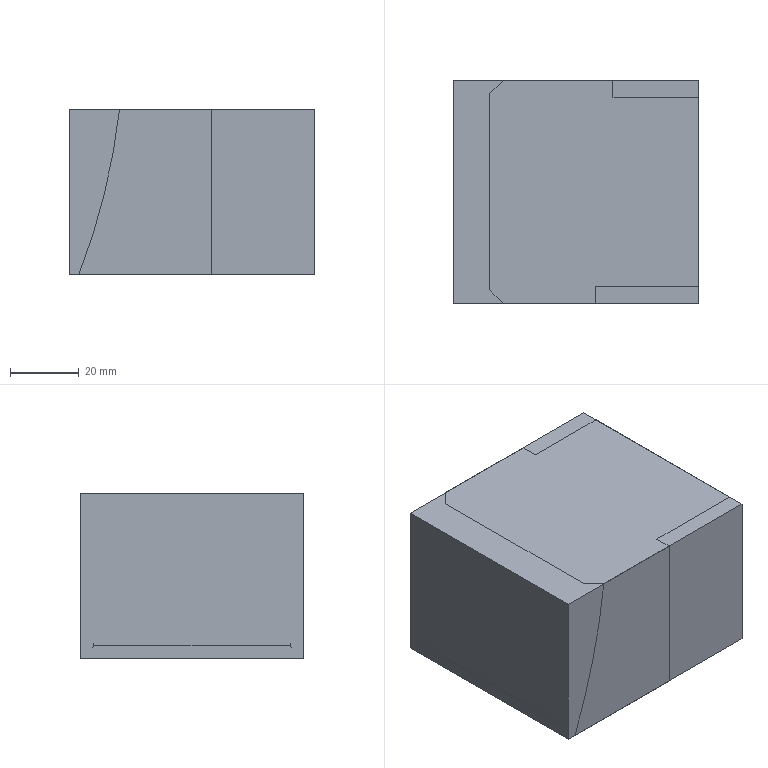NC program | NX | posted with a generic post | part box 71.51 x 65 x 48 mm
Whole program:
N10 G17 G21 G94 G90
(DRILLING_COPY_1 , TOOL : D6A45)
N12 T07 M6
N14 G54
N16 G17 G0 G90 X20. Y-16. B0. C0. S5000 M3
N18 G43 Z30. H7
N20 G94 G81 G98 Z-1. F250. R3.
N22 Y0.
N24 Y16.
N26 X-20.
N28 Y0.
N30 Y-16.
N32 G80
N34 G0 X-20. Y-16. Z30.
N36 M5
(DRILLING_COPY_COPY_1 , TOOL : 4.8ZT)
N38 T14 M6
N40 G54
N42 G17 G0 G90 X20. Y0. B0. C0. S2000 M3
N44 G43 Z30. H14
N46 G94 G83 G98 Z-13.442 F120. Q2. R3.
N48 X-20.
N50 G80
N52 G0 X-20. Y0. Z30.
N54 M5
(DRILLING_COPY_COPY_1_COPY , TOOL : 5.0JD)
N56 T15 M6
N58 G54
N60 G17 G0 G90 X20. Y0. B0. C0. S1000 M3
N62 G43 Z30. H15
N64 G94 G85 G98 Z-12. F50. R3.
N66 X-20.
N68 G80
N70 G0 X-20. Y0. Z30.
N72 M5
(DRILLING_COPY_COPY_1_COPY_1 , TOOL : 7.0ZT)
N74 T17 M6
N76 G54
N78 G17 G0 G90 X20. Y-16. B0. C0. S2000 M3
N80 G43 Z30. H17
N82 G94 G83 G98 Z-14.103 F200. Q2. R3.
N84 Y16.
N86 X-20.
N88 Y-16.
N90 G80
N92 G0 X-20. Y-16. Z30.
N94 M5
(ZLEVEL_PROFILE_COPY_COPY , TOOL : D10)
N96 T10 M6
N98 G54
N100 G17 G0 G90 X-34.486 Y-30.812 B0. C0. S9500 M3
N102 G43 Z30. H10
N104 Z-0.995
N106 G94 G1 X-33.099 Y-30.011 F1000.
N108 G3 X-32.599 Y-29.145 R1.
N110 G1 X-32.6 Y-23.776 F3500.
N112 Y23.009
N114 X-32.599 Y29.145
N116 G3 X-33.099 Y30.011 R1.
N118 G1 X-34.486 Y30.812
N120 G0 Z-1.99
N122 G1 X-33.099 Y30.011 F1000.
N124 G2 X-32.599 Y29.145 R1.
N126 G1 X-32.6 Y23.009 F3500.
N128 Y-23.776
N130 X-32.599 Y-29.145
N132 G2 X-33.099 Y-30.011 R1.
N134 G1 X-34.486 Y-30.812
N136 G0 Z-2.985
N138 G1 X-33.099 Y-30.011 F1000.
N140 G3 X-32.599 Y-29.145 R1.
N142 G1 X-32.6 Y-23.776 F3500.
N144 Y23.009
N146 X-32.599 Y29.145
N148 G3 X-33.099 Y30.011 R1.
N150 G1 X-34.486 Y30.812
N152 G0 Z-3.98
N154 G1 X-33.099 Y30.011 F1000.
N156 G2 X-32.599 Y29.145 R1.
N158 G1 X-32.6 Y23.009 F3500.
N160 Y-23.776
N162 X-32.599 Y-29.145
N164 G2 X-33.099 Y-30.011 R1.
N166 G1 X-34.486 Y-30.812
N168 G0 Z-4.975
N170 G1 X-33.099 Y-30.011 F1000.
N172 G3 X-32.599 Y-29.145 R1.
N174 G1 X-32.6 Y-23.776 F3500.
N176 Y23.009
N178 X-32.599 Y29.145
N180 G3 X-33.099 Y30.011 R1.
N182 G1 X-34.486 Y30.812
N184 G0 Z-5.97
N186 G1 X-33.099 Y30.011 F1000.
N188 G2 X-32.599 Y29.145 R1.
N190 G1 X-32.6 Y23.009 F3500.
N192 Y-23.776
N194 X-32.599 Y-29.145
N196 G2 X-33.099 Y-30.011 R1.
N198 G1 X-34.486 Y-30.812
N200 G0 Z-6.965
N202 G1 X-33.099 Y-30.011 F1000.
N204 G3 X-32.599 Y-29.145 R1.
N206 G1 X-32.6 Y-23.776 F3500.
N208 Y23.009
N210 X-32.599 Y29.145
N212 G3 X-33.099 Y30.011 R1.
N214 G1 X-34.486 Y30.812
N216 G0 Z-7.96
N218 G1 X-33.099 Y30.011 F1000.
N220 G2 X-32.599 Y29.145 R1.
N222 G1 X-32.6 Y23.009 F3500.
N224 Y-23.776
N226 X-32.599 Y-29.145
N228 G2 X-33.099 Y-30.011 R1.
N230 G1 X-34.486 Y-30.812
N232 G0 Z-8.955
N234 G1 X-33.099 Y-30.011 F1000.
N236 G3 X-32.599 Y-29.145 R1.
N238 G1 X-32.6 Y-23.776 F3500.
N240 Y23.009
N242 X-32.599 Y29.145
N244 G3 X-33.099 Y30.011 R1.
N246 G1 X-34.486 Y30.812
N248 G0 X-34.485 Y30.818 Z-9.95
N250 G1 X-33.097 Y30.013 F1000.
N252 G2 X-32.599 Y29.145 R1.
N254 G1 X-32.601 Y28.378 F3500.
N256 X-32.6 Y23.009
N258 Y-23.776
N260 X-32.601 Y-28.378
N262 X-32.599 Y-29.145
N264 G2 X-33.097 Y-30.013 R1.
N266 G1 X-34.485 Y-30.818
N268 G0 Y-30.819 Z-10.945
N270 G1 X-33.097 Y-30.013 F1000.
N272 G3 X-32.599 Y-29.145 R1.
N274 G1 X-32.601 Y-28.378 F3500.
N276 X-32.6 Y-23.776
N278 Y23.009
N280 X-32.601 Y28.378
N282 X-32.599 Y29.145
N284 G3 X-33.097 Y30.013 R1.
N286 G1 X-34.485 Y30.819
N288 G0 X-34.484 Z-11.94
N290 G1 X-33.097 Y30.013 F1000.
N292 G2 X-32.599 Y29.145 R1.
N294 G1 X-32.602 Y28.378 F3500.
N296 X-32.6 Y23.009
N298 Y-23.776
N300 X-32.602 Y-28.378
N302 X-32.599 Y-29.145
N304 G2 X-33.097 Y-30.013 R1.
N306 G1 X-34.484 Y-30.819
N308 G0 X-34.486 Y-30.812 Z-12.935
N310 G1 X-33.099 Y-30.011 F1000.
N312 G3 X-32.599 Y-29.145 R1.
N314 G1 X-32.6 Y-23.776 F3500.
N316 Y23.009
N318 X-32.602 Y28.378
N320 X-32.599 Y29.145
N322 G3 X-33.097 Y30.013 R1.
N324 G1 X-34.484 Y30.82
N326 G0 Z-13.93
N328 G1 X-33.097 Y30.013 F1000.
N330 G2 X-32.599 Y29.145 R1.
N332 G1 X-32.602 Y28.378 F3500.
N334 X-32.6 Y23.009
N336 Y-23.776
N338 X-32.599 Y-29.145
N340 G2 X-33.099 Y-30.011 R1.
N342 G1 X-34.486 Y-30.812
N344 G0 Z-14.925
N346 G1 X-33.099 Y-30.011 F1000.
N348 G3 X-32.599 Y-29.145 R1.
N350 G1 X-32.6 Y-23.776 F3500.
N352 Y23.009
N354 X-32.602 Y28.378
N356 X-32.599 Y29.145
N358 G3 X-33.097 Y30.013 R1.
N360 G1 X-34.484 Y30.82
N362 G0 Y30.821 Z-15.92
N364 G1 X-33.096 Y30.013 F1000.
N366 G2 X-32.599 Y29.145 R1.
N368 G1 X-32.602 Y28.378 F3500.
N370 X-32.6 Y23.009
N372 Y-23.776
N374 X-32.599 Y-29.145
N376 G2 X-33.099 Y-30.011 R1.
N378 G1 X-34.486 Y-30.812
N380 G0 Z-16.915
N382 G1 X-33.099 Y-30.011 F1000.
N384 G3 X-32.6 Y-29.145 R1.
N386 G1 Y-23.776 F3500.
N388 Y23.009
N390 X-32.602 Y28.378
N392 X-32.6 Y29.145
N394 G3 X-33.096 Y30.013 R1.
N396 G1 X-34.484 Y30.821
N398 G0 Y30.822 Z-17.91
N400 G1 X-33.096 Y30.013 F1000.
N402 G2 X-32.6 Y29.145 R1.
N404 G1 X-32.602 Y28.378 F3500.
N406 X-32.6 Y23.009
N408 Y-23.776
N410 Y-29.145
N412 G2 X-33.099 Y-30.011 R1.
N414 G1 X-34.486 Y-30.812
N416 G0 Z-18.905
N418 G1 X-33.099 Y-30.011 F1000.
N420 G3 X-32.6 Y-29.145 R1.
N422 G1 Y-23.776 F3500.
N424 Y23.009
N426 Y29.145
N428 G3 X-33.099 Y30.011 R1.
N430 G1 X-34.486 Y30.812
N432 G0 Z-19.9
N434 G1 X-33.1 Y30.011 F1000.
N436 G2 X-32.6 Y29.145 R1.
N438 G1 Y23.009 F3500.
N440 Y-23.776
N442 Y-29.145
N444 G2 X-33.1 Y-30.011 R1.
N446 G1 X-34.486 Y-30.812
N448 G0 Z-20.895
N450 G1 X-33.1 Y-30.011 F1000.
N452 G3 X-32.6 Y-29.145 R1.
N454 G1 Y-23.776 F3500.
N456 Y23.009
N458 Y29.145
N460 G3 X-33.1 Y30.011 R1.
N462 G1 X-34.486 Y30.812
N464 G0 Z-21.89
N466 G1 X-33.1 Y30.011 F1000.
N468 G2 X-32.6 Y29.145 R1.
N470 G1 Y23.009 F3500.
N472 Y-23.776
N474 Y-29.145
N476 G2 X-33.1 Y-30.011 R1.
N478 G1 X-34.486 Y-30.812
N480 G0 Z-22.885
N482 G1 X-33.1 Y-30.011 F1000.
N484 G3 X-32.6 Y-29.145 R1.
N486 G1 Y-23.776 F3500.
N488 Y23.009
N490 Y29.145
N492 G3 X-33.1 Y30.011 R1.
N494 G1 X-34.486 Y30.812
N496 G0 Z-23.88
N498 G1 X-33.1 Y30.011 F1000.
N500 G2 X-32.6 Y29.145 R1.
N502 G1 Y23.009 F3500.
N504 Y-23.776
N506 Y-29.145
N508 G2 X-33.1 Y-30.011 R1.
N510 G1 X-34.486 Y-30.812
N512 G0 X-34.484 Y-30.825 Z-24.875
N514 G1 X-33.095 Y-30.014 F1000.
N516 G3 X-32.6 Y-29.145 R1.
N518 G1 X-32.603 Y-28.378 F3500.
N520 X-32.6 Y-23.776
N522 Y23.009
N524 X-32.601 Y23.776
N526 X-32.6 Y29.145
N528 G3 X-33.1 Y30.011 R1.
N530 G1 X-34.486 Y30.812
N532 G0 X-34.484 Y30.825 Z-25.87
N534 G1 X-33.095 Y30.014 F1000.
N536 G2 X-32.6 Y29.145 R1.
N538 G1 X-32.604 Y28.378 F3500.
N540 X-32.6 Y23.009
N542 Y-23.776
N544 Y-24.034
N546 X-32.604 Y-28.378
N548 X-32.6 Y-29.145
N550 G2 X-33.095 Y-30.014 R1.
N552 G1 X-34.484 Y-30.825
N554 G0 X-34.486 Y-30.812 Z-26.865
N556 G1 X-33.1 Y-30.011 F1000.
N558 G3 X-32.6 Y-29.145 R1.
N560 G1 Y-23.776 F3500.
N562 Y23.009
N564 X-32.604 Y28.378
N566 X-32.6 Y29.145
N568 G3 X-33.095 Y30.014 R1.
N570 G1 X-34.484 Y30.825
N572 G0 X-34.483 Y30.826 Z-27.86
N574 G1 X-33.095 Y30.014 F1000.
N576 G2 X-32.6 Y29.145 R1.
N578 G1 X-32.604 Y28.378 F3500.
N580 X-32.6 Y23.009
N582 Y-23.776
N584 Y-29.145
N586 G2 X-33.1 Y-30.011 R1.
N588 G1 X-34.486 Y-30.812
N590 G0 Z-28.855
N592 G1 X-33.1 Y-30.011 F1000.
N594 G3 X-32.6 Y-29.145 R1.
N596 G1 Y-23.776 F3500.
N598 Y23.009
N600 X-32.604 Y28.378
N602 X-32.6 Y29.145
N604 G3 X-33.095 Y30.014 R1.
N606 G1 X-34.483 Y30.826
N608 G0 Y30.827 Z-29.85
N610 G1 X-33.095 Y30.014 F1000.
N612 G2 X-32.6 Y29.145 R1.
N614 G1 X-32.604 Y28.378 F3500.
N616 X-32.6 Y23.009
N618 Y-23.776
N620 X-32.604 Y-24.783
N622 X-32.6 Y-29.145
N624 G2 X-33.099 Y-30.012 R1.
N626 G1 X-34.486 Y-30.814
N628 G0 Z30.
(ZLEVEL_PROFILE_COPY_COPY_COPY_1 , TOOL : D10)
N630 X34.486 Y30.812
N632 Z-0.994
N634 G1 X33.099 Y30.011 F1000.
N636 G3 X32.599 Y29.145 R1.
N638 G1 X32.6 Y23.009 F3500.
N640 Y-23.776
N642 X32.541 Y-24.774
N644 X32.6 Y-24.831
N646 X32.599 Y-29.145
N648 G3 X33.099 Y-30.011 R1.
N650 G1 X34.486 Y-30.812
N652 G0 Z-1.988
N654 G1 X33.099 Y-30.011 F1000.
N656 G2 X32.599 Y-29.145 R1.
N658 G1 X32.6 Y-24.831 F3500.
N660 X32.541 Y-24.774
N662 X32.6 Y-23.776
N664 Y23.009
N666 X32.599 Y29.145
N668 G2 X33.099 Y30.011 R1.
N670 G1 X34.486 Y30.812
N672 G0 Z-2.982
N674 G1 X33.099 Y30.011 F1000.
N676 G3 X32.599 Y29.145 R1.
N678 G1 X32.6 Y23.009 F3500.
N680 Y-23.776
N682 X32.541 Y-24.774
N684 X32.6 Y-24.831
N686 X32.599 Y-29.145
N688 G3 X33.099 Y-30.011 R1.
N690 G1 X34.486 Y-30.812
N692 G0 Z-3.976
N694 G1 X33.099 Y-30.011 F1000.
N696 G2 X32.599 Y-29.145 R1.
N698 G1 X32.6 Y-24.831 F3500.
N700 X32.541 Y-24.774
N702 X32.6 Y-23.776
N704 Y23.009
N706 X32.599 Y29.145
N708 G2 X33.099 Y30.011 R1.
N710 G1 X34.486 Y30.812
N712 G0 Z-4.97
N714 G1 X33.099 Y30.011 F1000.
N716 G3 X32.599 Y29.145 R1.
N718 G1 X32.6 Y23.009 F3500.
N720 Y-23.776
N722 X32.541 Y-24.774
N724 X32.6 Y-24.831
N726 X32.599 Y-29.145
N728 G3 X33.099 Y-30.011 R1.
N730 G1 X34.486 Y-30.812
N732 G0 Z-5.964
N734 G1 X33.099 Y-30.011 F1000.
N736 G2 X32.599 Y-29.145 R1.
N738 G1 X32.6 Y-24.831 F3500.
N740 X32.541 Y-24.774
N742 X32.6 Y-23.776
N744 Y23.009
N746 X32.599 Y29.145
N748 G2 X33.099 Y30.011 R1.
N750 G1 X34.486 Y30.812
N752 G0 Z-6.958
N754 G1 X33.099 Y30.011 F1000.
N756 G3 X32.599 Y29.145 R1.
N758 G1 X32.6 Y23.009 F3500.
N760 Y-23.776
N762 X32.541 Y-24.774
N764 X32.6 Y-24.831
N766 X32.599 Y-29.145
N768 G3 X33.099 Y-30.011 R1.
N770 G1 X34.486 Y-30.812
N772 G0 Z-7.952
N774 G1 X33.099 Y-30.011 F1000.
N776 G2 X32.599 Y-29.145 R1.
N778 G1 X32.6 Y-24.831 F3500.
N780 X32.541 Y-24.774
N782 X32.6 Y-23.776
N784 Y23.009
N786 X32.599 Y29.145
N788 G2 X33.099 Y30.011 R1.
N790 G1 X34.486 Y30.812
N792 G0 Z-8.946
N794 G1 X33.099 Y30.011 F1000.
N796 G3 X32.599 Y29.145 R1.
N798 G1 X32.6 Y23.009 F3500.
N800 Y-23.776
N802 X32.541 Y-24.774
N804 X32.6 Y-24.831
N806 X32.599 Y-29.145
N808 G3 X33.099 Y-30.011 R1.
N810 G1 X34.486 Y-30.812
N812 G0 Z-9.94
N814 G1 X33.099 Y-30.011 F1000.
N816 G2 X32.599 Y-29.145 R1.
N818 G1 X32.6 Y-24.831 F3500.
N820 X32.541 Y-24.774
N822 X32.6 Y-23.776
N824 Y23.009
N826 X32.599 Y29.145
N828 G2 X33.099 Y30.011 R1.
N830 G1 X34.486 Y30.812
N832 G0 Z-10.934
N834 G1 X33.099 Y30.011 F1000.
N836 G3 X32.599 Y29.145 R1.
N838 G1 X32.6 Y23.009 F3500.
N840 Y-23.776
N842 X32.541 Y-24.774
N844 X32.6 Y-24.831
N846 X32.599 Y-29.145
N848 G3 X33.099 Y-30.011 R1.
N850 G1 X34.486 Y-30.812
N852 G0 Z-11.928
N854 G1 X33.099 Y-30.011 F1000.
N856 G2 X32.599 Y-29.145 R1.
N858 G1 X32.6 Y-24.831 F3500.
N860 X32.541 Y-24.774
N862 X32.6 Y-23.776
N864 Y23.009
N866 X32.599 Y29.145
N868 G2 X33.099 Y30.011 R1.
N870 G1 X34.486 Y30.812
N872 G0 Z-12.922
N874 G1 X33.099 Y30.011 F1000.
N876 G3 X32.599 Y29.145 R1.
N878 G1 X32.6 Y23.009 F3500.
N880 Y-23.776
N882 X32.541 Y-24.774
N884 X32.6 Y-24.831
N886 X32.599 Y-29.145
N888 G3 X33.099 Y-30.011 R1.
N890 G1 X34.486 Y-30.812
N892 G0 Z-13.916
N894 G1 X33.099 Y-30.011 F1000.
N896 G2 X32.6 Y-29.145 R1.
N898 G1 Y-24.831 F3500.
N900 X32.541 Y-24.774
N902 X32.6 Y-23.776
N904 Y23.009
N906 Y29.145
N908 G2 X33.099 Y30.011 R1.
N910 G1 X34.486 Y30.812
N912 G0 Z-14.91
N914 G1 X33.099 Y30.011 F1000.
N916 G3 X32.6 Y29.145 R1.
N918 G1 Y23.009 F3500.
N920 Y-23.776
N922 X32.541 Y-24.774
N924 X32.6 Y-24.831
N926 Y-29.145
N928 G3 X33.099 Y-30.011 R1.
N930 G1 X34.486 Y-30.812
N932 G0 Z-15.904
N934 G1 X33.099 Y-30.011 F1000.
N936 G2 X32.6 Y-29.145 R1.
N938 G1 Y-24.831 F3500.
N940 X32.541 Y-24.774
N942 X32.6 Y-23.776
N944 Y23.009
N946 Y29.145
N948 G2 X33.099 Y30.011 R1.
N950 G1 X34.486 Y30.812
N952 G0 Z-16.898
N954 G1 X33.1 Y30.011 F1000.
N956 G3 X32.6 Y29.145 R1.
N958 G1 Y23.009 F3500.
N960 Y-23.776
N962 X32.541 Y-24.774
N964 X32.6 Y-24.831
N966 Y-29.145
N968 G3 X33.099 Y-30.011 R1.
N970 G1 X34.486 Y-30.812
N972 G0 Z-17.892
N974 G1 X33.099 Y-30.011 F1000.
N976 G2 X32.6 Y-29.145 R1.
N978 G1 Y-24.831 F3500.
N980 X32.541 Y-24.774
N982 X32.6 Y-23.776
N984 Y23.009
N986 Y29.145
N988 G2 X33.1 Y30.011 R1.
N990 G1 X34.486 Y30.812
N992 G0 Z-18.886
N994 G1 X33.1 Y30.011 F1000.
N996 G3 X32.6 Y29.145 R1.
N998 G1 Y23.009 F3500.
N1000 Y-23.776
N1002 X32.541 Y-24.774
N1004 X32.6 Y-24.831
N1006 Y-29.145
N1008 G3 X33.099 Y-30.011 R1.
N1010 G1 X34.486 Y-30.812
N1012 G0 Z-19.88
N1014 G1 X33.099 Y-30.011 F1000.
N1016 G2 X32.6 Y-29.145 R1.
N1018 G1 Y-24.831 F3500.
N1020 X32.541 Y-24.774
N1022 X32.6 Y-23.776
N1024 Y23.009
N1026 Y29.145
N1028 G2 X33.1 Y30.011 R1.
N1030 G1 X34.486 Y30.812
N1032 G0 Z-20.874
N1034 G1 X33.1 Y30.011 F1000.
N1036 G3 X32.6 Y29.145 R1.
N1038 G1 Y23.009 F3500.
N1040 Y-23.776
N1042 X32.541 Y-24.774
N1044 X32.601 Y-24.831
N1046 X32.6 Y-29.145
N1048 G3 X33.099 Y-30.011 R1.
N1050 G1 X34.486 Y-30.812
N1052 G0 Z-21.868
N1054 G1 X33.1 Y-30.011 F1000.
N1056 G2 X32.6 Y-29.145 R1.
N1058 G1 X32.601 Y-24.831 F3500.
N1060 X32.541 Y-24.774
N1062 X32.6 Y-23.776
N1064 Y23.009
N1066 Y29.145
N1068 G2 X33.1 Y30.011 R1.
N1070 G1 X34.486 Y30.812
N1072 G0 Z-22.862
N1074 G1 X33.1 Y30.011 F1000.
N1076 G3 X32.6 Y29.145 R1.
N1078 G1 Y23.009 F3500.
N1080 Y-23.776
N1082 X32.541 Y-24.774
N1084 X32.601 Y-24.831
N1086 X32.6 Y-29.145
N1088 G3 X33.1 Y-30.011 R1.
N1090 G1 X34.486 Y-30.812
N1092 G0 Z-23.856
N1094 G1 X33.1 Y-30.011 F1000.
N1096 G2 X32.6 Y-29.145 R1.
N1098 G1 X32.601 Y-24.831 F3500.
N1100 X32.541 Y-24.774
N1102 X32.6 Y-23.776
N1104 Y23.009
N1106 Y29.145
N1108 G2 X33.1 Y30.011 R1.
N1110 G1 X34.486 Y30.812
N1112 G0 Z-24.85
N1114 G1 X33.1 Y30.011 F1000.
N1116 G3 X32.6 Y29.145 R1.
N1118 G1 Y23.009 F3500.
N1120 Y-23.776
N1122 X32.548 Y-24.728
N1124 X32.601 Y-24.783
N1126 X32.6 Y-29.145
N1128 G3 X33.1 Y-30.011 R1.
N1130 G1 X34.486 Y-30.812
N1132 G0 Z30.
N1134 M5
(ZLEVEL_PROFILE_COPY_COPY_COPY_COPY , TOOL : D10JING)
N1136 T11 M6
N1138 G54
N1140 G17 G0 G90 X34.37 Y30.869 B0. C0. S9500 M3
N1142 G43 Z30. H11
N1144 Z-9.5
N1146 G94 G1 Z-12.5 F1000.
N1148 X32.997 Y30.076
N1150 G3 X32.498 Y29.209 R1.
N1152 G1 X32.5 Y23.444 F1500.
N1154 Y-24.
N1156 X32.446 Y-24.734
N1158 X32.503 Y-24.732
N1160 X32.498 Y-24.789
N1162 Y-29.209
N1164 G3 X32.998 Y-30.075 R1.
N1166 G1 X34.37 Y-30.868
N1168 Z-9.5
N1170 G0 X34.372 Y30.868 Z-22.
N1172 G1 Z-25. F1000.
N1174 X32.999 Y30.075
N1176 G3 X32.499 Y29.209 R1.
N1178 G1 X32.5 Y23.444 F1500.
N1180 Y-24.
N1182 X32.446 Y-24.734
N1184 X32.504 Y-24.731
N1186 X32.5 Y-24.79
N1188 X32.499 Y-29.209
N1190 G3 X32.999 Y-30.075 R1.
N1192 G1 X34.371 Y-30.868
N1194 Z-22.
N1196 G0 Z30.
N1198 X-34.368 Y-30.883
N1200 Z-9.5
N1202 G1 Z-12.5 F1000.
N1204 X-32.994 Y-30.078
N1206 G3 X-32.499 Y-29.209 R1.
N1208 G1 X-32.502 Y-28.825 F1500.
N1210 X-32.5 Y-23.965
N1212 Y23.444
N1214 X-32.502 Y28.825
N1216 X-32.499 Y29.209
N1218 G3 X-32.994 Y30.078 R1.
N1220 G1 X-34.368 Y30.883
N1222 Z-9.5
N1224 G0 X-34.373 Y-30.867 Z-22.
N1226 G1 Z-25. F1000.
N1228 X-33.001 Y-30.075
N1230 G3 X-32.501 Y-29.209 R1.
N1232 G1 X-32.5 Y-23.965 F1500.
N1234 Y23.444
N1236 X-32.503 Y24.213
N1238 Y28.825
N1240 X-32.501 Y29.209
N1242 G3 X-32.995 Y30.079 R1.
N1244 G1 X-34.369 Y30.885
N1246 Z-22.
N1248 G0 X-34.373 Y-30.867 Z-27.
N1250 G1 Z-30. F1000.
N1252 X-33.002 Y-30.075
N1254 G3 X-32.501 Y-29.209 R1.
N1256 G1 X-32.5 Y-23.965 F1500.
N1258 Y23.444
N1260 X-32.504 Y24.213
N1262 Y28.825
N1264 X-32.501 Y29.209
N1266 G3 X-32.995 Y30.079 R1.
N1268 G1 X-34.37 Y30.885
N1270 Z-27.
N1272 G0 Z30.
N1274 M5
(ZLEVEL_PROFILE_1_COPY_1_COPY_COPY , TOOL : D6A45)
N1276 T07 M6
N1278 G54
N1280 G17 G0 G90 X19.697 Y-17.307 B0. C0. S9500 M3
N1282 G43 Z30. H7
N1284 Z0.
N1286 G94 G1 Z-1. F1000.
N1288 X19.48 Y-18.241
N1290 G3 X20. Y-18.541 R0.6
N1292 G1 X20.008
N1294 G3 X22.541 Y-15.992 R2.541
N1296 X20. Y-18.541 R-2.541
N1298 X20.52 Y-18.241 R0.6
N1300 G1 X20.303 Y-17.307
N1302 Z0.
N1304 G0 Z30.
N1306 Y17.307
N1308 Z0.
N1310 G1 Z-1.
N1312 X20.52 Y18.241
N1314 G3 X20. Y18.541 R0.6
N1316 X17.459 Y16. R2.541
N1318 X20. Y18.541 R-2.541
N1320 X19.48 Y18.241 R0.6
N1322 G1 X19.697 Y17.307
N1324 Z0.
N1326 G0 Z30.
N1328 X-20.315 Y0.132
N1330 Z0.
N1332 G1 Z-1.
N1334 X-21.241 Y0.52
N1336 G3 X-21.541 Y0. R0.6
N1338 X-20. Y-1.541 R1.541
N1340 X-21.541 Y0. R-1.541
N1342 X-21.241 Y-0.52 R0.6
N1344 G1 X-20.315 Y-0.132
N1346 Z0.
N1348 G0 Z30.
N1350 X-19.697 Y17.307
N1352 Z0.
N1354 G1 Z-1.
N1356 X-19.48 Y18.241
N1358 G3 X-20. Y18.541 R0.6
N1360 G1 X-20.007
N1362 G3 X-22.541 Y15.993 R2.541
N1364 X-20. Y18.541 R-2.541
N1366 X-20.52 Y18.241 R0.6
N1368 G1 X-20.303 Y17.307
N1370 Z0.
N1372 G0 Z30.
N1374 Y-17.307
N1376 Z0.
N1378 G1 Z-1.
N1380 X-20.52 Y-18.241
N1382 G3 X-20. Y-18.541 R0.6
N1384 X-17.459 Y-16. R2.541
N1386 X-20. Y-18.541 R-2.541
N1388 X-19.48 Y-18.241 R0.6
N1390 G1 X-19.697 Y-17.307
N1392 Z0.
N1394 G0 Z30.
N1396 X20.315 Y-0.132
N1398 Z0.
N1400 G1 Z-1.
N1402 X21.241 Y-0.52
N1404 G3 X21.541 Y0. R0.6
N1406 X20. Y1.541 R1.541
N1408 X21.541 Y0. R-1.541
N1410 X21.241 Y0.52 R0.6
N1412 G1 X20.315 Y0.132
N1414 Z0.
N1416 G0 Z30.
N1418 X28.421 Y-25.953
N1420 Z0.
N1422 G1 Z-1.
N1424 X28.02 Y-25.259
N1426 G3 X27.501 Y-24.959 R0.6
N1428 G1 X-27.501
N1430 G2 X-28.459 Y-24.001 R0.958
N1432 G1 Y24.001
N1434 G2 X-27.501 Y24.959 R0.958
N1436 G1 X27.501
N1438 G2 X28.459 Y24.001 R0.958
N1440 G1 Y-24.001
N1442 G2 X27.501 Y-24.959 R0.958
N1444 G3 X26.981 Y-25.259 R0.6
N1446 G1 X26.461 Y-26.159
N1448 Z0.
N1450 G0 Z30.
N1452 M5
N1454 M2